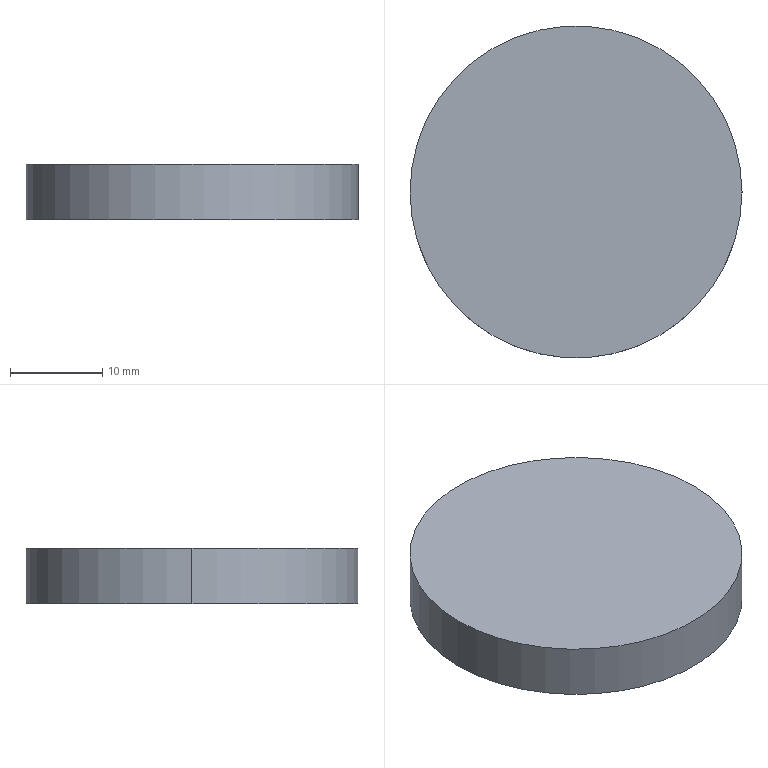Part | SolidWorks | features BaseBody 1 | 1 solid | 4 faces | box 36 x 36 x 6 mm | volume 6107 mm3 | cylinder 2 | plane 2 | commonest cylinder face diameters 36 x2
STEP:
#1=CARTESIAN_POINT('',(18.,0.,-3.));
#2=VERTEX_POINT('',#1);
#3=CARTESIAN_POINT('',(-18.,0.,-3.));
#4=VERTEX_POINT('',#3);
#5=CARTESIAN_POINT('',(0.,0.,-3.));
#6=DIRECTION('',(0.,0.,1.));
#7=DIRECTION('',(1.,0.,0.));
#8=AXIS2_PLACEMENT_3D('',#5,#6,#7);
#9=CIRCLE('',#8,18.);
#10=EDGE_CURVE('',#2,#4,#9,.T.);
#11=ORIENTED_EDGE('',*,*,#10,.T.);
#12=CARTESIAN_POINT('',(-18.,0.,3.));
#13=VERTEX_POINT('',#12);
#14=CARTESIAN_POINT('',(-18.,0.,-3.));
#15=DIRECTION('',(0.,0.,1.));
#16=VECTOR('',#15,1000.);
#17=LINE('',#14,#16);
#18=EDGE_CURVE('',#4,#13,#17,.T.);
#19=ORIENTED_EDGE('',*,*,#18,.T.);
#20=CARTESIAN_POINT('',(18.,0.,3.));
#21=VERTEX_POINT('',#20);
#22=CARTESIAN_POINT('',(0.,0.,3.));
#23=DIRECTION('',(0.,0.,1.));
#24=DIRECTION('',(1.,0.,0.));
#25=AXIS2_PLACEMENT_3D('',#22,#23,#24);
#26=CIRCLE('',#25,18.);
#27=EDGE_CURVE('',#21,#13,#26,.T.);
#28=ORIENTED_EDGE('',*,*,#27,.F.);
#29=CARTESIAN_POINT('',(18.,0.,-3.));
#30=DIRECTION('',(0.,0.,1.));
#31=VECTOR('',#30,1000.);
#32=LINE('',#29,#31);
#33=EDGE_CURVE('',#2,#21,#32,.T.);
#34=ORIENTED_EDGE('',*,*,#33,.F.);
#35=EDGE_LOOP('',(#11,#19,#28,#34));
#36=FACE_OUTER_BOUND('',#35,.T.);
#37=CARTESIAN_POINT('',(0.,0.,-3.));
#38=DIRECTION('',(0.,0.,1.));
#39=DIRECTION('',(1.,0.,0.));
#40=AXIS2_PLACEMENT_3D('',#37,#38,#39);
#41=CYLINDRICAL_SURFACE('',#40,18.);
#42=ADVANCED_FACE('',(#36),#41,.T.);
#43=ORIENTED_EDGE('',*,*,#27,.T.);
#44=CARTESIAN_POINT('',(0.,0.,3.));
#45=DIRECTION('',(0.,0.,1.));
#46=DIRECTION('',(1.,0.,0.));
#47=AXIS2_PLACEMENT_3D('',#44,#45,#46);
#48=CIRCLE('',#47,18.);
#49=EDGE_CURVE('',#13,#21,#48,.T.);
#50=ORIENTED_EDGE('',*,*,#49,.T.);
#51=EDGE_LOOP('',(#43,#50));
#52=FACE_OUTER_BOUND('',#51,.T.);
#53=CARTESIAN_POINT('',(0.,0.,3.));
#54=DIRECTION('',(0.,0.,1.));
#55=DIRECTION('',(1.,0.,0.));
#56=AXIS2_PLACEMENT_3D('',#53,#54,#55);
#57=PLANE('',#56);
#58=ADVANCED_FACE('',(#52),#57,.T.);
#59=ORIENTED_EDGE('',*,*,#18,.F.);
#60=CARTESIAN_POINT('',(0.,0.,-3.));
#61=DIRECTION('',(0.,0.,1.));
#62=DIRECTION('',(1.,0.,0.));
#63=AXIS2_PLACEMENT_3D('',#60,#61,#62);
#64=CIRCLE('',#63,18.);
#65=EDGE_CURVE('',#4,#2,#64,.T.);
#66=ORIENTED_EDGE('',*,*,#65,.T.);
#67=ORIENTED_EDGE('',*,*,#33,.T.);
#68=ORIENTED_EDGE('',*,*,#49,.F.);
#69=EDGE_LOOP('',(#59,#66,#67,#68));
#70=FACE_OUTER_BOUND('',#69,.T.);
#71=CARTESIAN_POINT('',(0.,0.,-3.));
#72=DIRECTION('',(0.,0.,1.));
#73=DIRECTION('',(1.,0.,0.));
#74=AXIS2_PLACEMENT_3D('',#71,#72,#73);
#75=CYLINDRICAL_SURFACE('',#74,18.);
#76=ADVANCED_FACE('',(#70),#75,.T.);
#77=ORIENTED_EDGE('',*,*,#10,.F.);
#78=ORIENTED_EDGE('',*,*,#65,.F.);
#79=EDGE_LOOP('',(#77,#78));
#80=FACE_OUTER_BOUND('',#79,.T.);
#81=CARTESIAN_POINT('',(0.,0.,-3.));
#82=DIRECTION('',(0.,0.,1.));
#83=DIRECTION('',(1.,0.,0.));
#84=AXIS2_PLACEMENT_3D('',#81,#82,#83);
#85=PLANE('',#84);
#86=ADVANCED_FACE('',(#80),#85,.F.);
#87=CLOSED_SHELL('',(#42,#58,#76,#86));
#88=MANIFOLD_SOLID_BREP('',#87);
#89=CARTESIAN_POINT('',(0.,0.,0.));
#90=DIRECTION('',(0.,0.,1.));
#91=DIRECTION('',(1.,0.,0.));
#92=AXIS2_PLACEMENT_3D('',#89,#90,#91);
#93=(LENGTH_UNIT()NAMED_UNIT(*)SI_UNIT(.MILLI.,.METRE.));
#94=UNCERTAINTY_MEASURE_WITH_UNIT(LENGTH_MEASURE(0.00001),#93,'','');
#95=(NAMED_UNIT(*)PLANE_ANGLE_UNIT()SI_UNIT($,.RADIAN.));
#96=(NAMED_UNIT(*)SI_UNIT($,.STERADIAN.)SOLID_ANGLE_UNIT());
#97=(GEOMETRIC_REPRESENTATION_CONTEXT(3)GLOBAL_UNCERTAINTY_ASSIGNED_CONTEXT((#94))GLOBAL_UNIT_ASSIGNED_CONTEXT((#93,#95,#96))REPRESENTATION_CONTEXT('',''));
#98=ADVANCED_BREP_SHAPE_REPRESENTATION('',(#88,#92),#97);